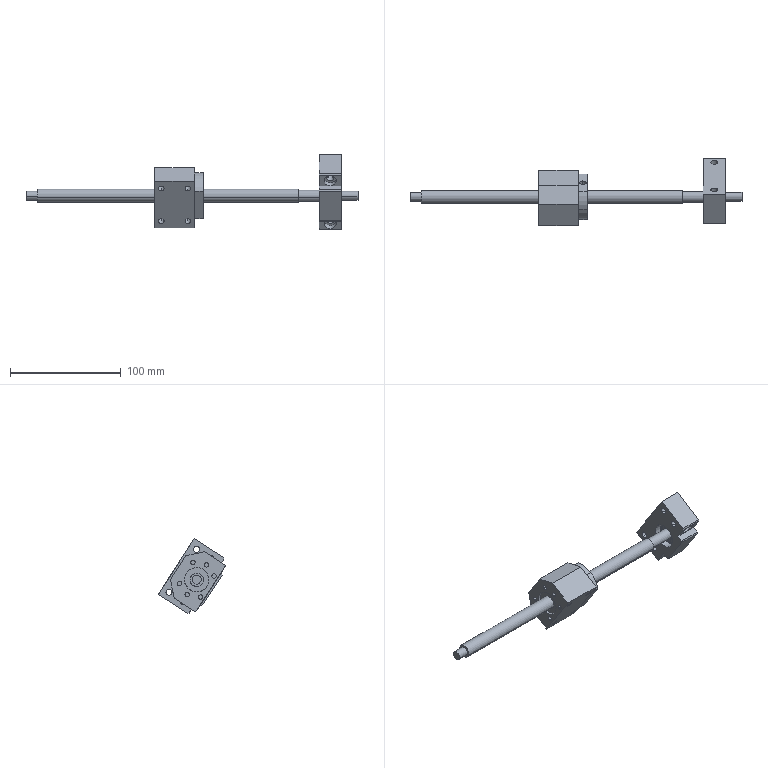Part | SolidWorks | 4 solids | 231 faces | box 300 x 60.871 x 67.503 mm | volume 121134 mm3 | cylinder 105 | plane 50 | cone 44 | torus 32 | commonest cylinder face diameters 5.5 x16 4 x12 4.8 x12 5 x8 8 x6 22 x6